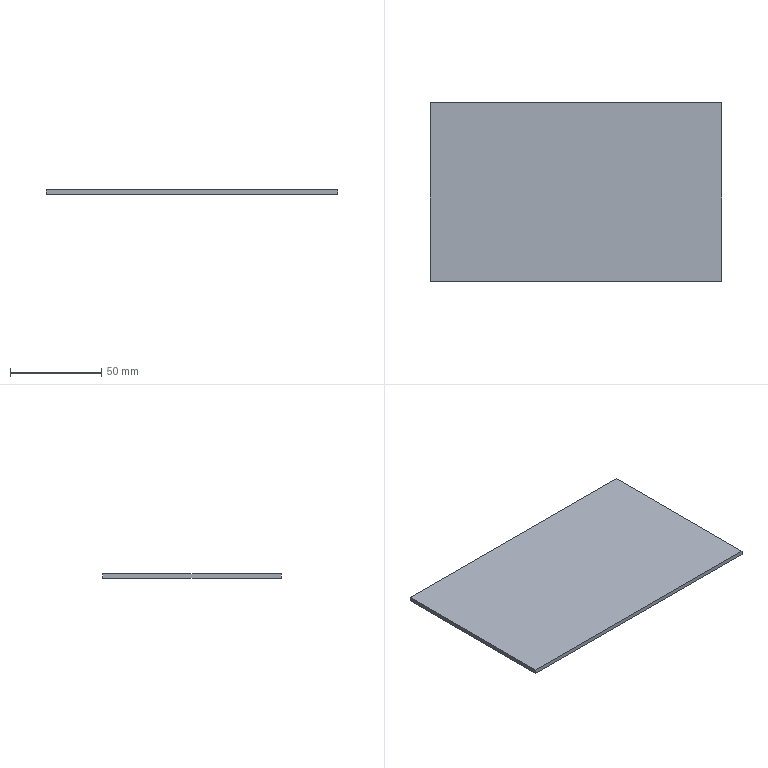Part | SolidWorks | features FlatPattern 1, SMBaseFlange 1, SheetMetal 1 | 1 solid | 6 faces | box 160 x 97.8 x 2.3 mm | volume 35990 mm3 | plane 6
STEP:
#1=CARTESIAN_POINT('',(0.,0.,0.));
#2=VERTEX_POINT('',#1);
#3=CARTESIAN_POINT('',(0.,-97.8,0.));
#4=VERTEX_POINT('',#3);
#5=CARTESIAN_POINT('',(0.,0.,0.));
#6=DIRECTION('',(0.,-1.,0.));
#7=VECTOR('',#6,1000.);
#8=LINE('',#5,#7);
#9=EDGE_CURVE('',#2,#4,#8,.T.);
#10=ORIENTED_EDGE('',*,*,#9,.F.);
#11=CARTESIAN_POINT('',(0.,0.,-2.3));
#12=VERTEX_POINT('',#11);
#13=CARTESIAN_POINT('',(0.,0.,-2.3));
#14=DIRECTION('',(0.,0.,1.));
#15=VECTOR('',#14,1000.);
#16=LINE('',#13,#15);
#17=EDGE_CURVE('',#12,#2,#16,.T.);
#18=ORIENTED_EDGE('',*,*,#17,.F.);
#19=CARTESIAN_POINT('',(0.,-97.8,-2.3));
#20=VERTEX_POINT('',#19);
#21=CARTESIAN_POINT('',(0.,0.,-2.3));
#22=DIRECTION('',(0.,-1.,0.));
#23=VECTOR('',#22,1000.);
#24=LINE('',#21,#23);
#25=EDGE_CURVE('',#12,#20,#24,.T.);
#26=ORIENTED_EDGE('',*,*,#25,.T.);
#27=CARTESIAN_POINT('',(0.,-97.8,-2.3));
#28=DIRECTION('',(0.,0.,1.));
#29=VECTOR('',#28,1000.);
#30=LINE('',#27,#29);
#31=EDGE_CURVE('',#20,#4,#30,.T.);
#32=ORIENTED_EDGE('',*,*,#31,.T.);
#33=EDGE_LOOP('',(#10,#18,#26,#32));
#34=FACE_OUTER_BOUND('',#33,.T.);
#35=CARTESIAN_POINT('',(0.,0.,-2.3));
#36=DIRECTION('',(-1.,0.,0.));
#37=DIRECTION('',(0.,-1.,0.));
#38=AXIS2_PLACEMENT_3D('',#35,#36,#37);
#39=PLANE('',#38);
#40=ADVANCED_FACE('',(#34),#39,.T.);
#41=CARTESIAN_POINT('',(160.,0.,0.));
#42=VERTEX_POINT('',#41);
#43=CARTESIAN_POINT('',(0.,0.,0.));
#44=DIRECTION('',(-1.,0.,0.));
#45=VECTOR('',#44,1000.);
#46=LINE('',#43,#45);
#47=EDGE_CURVE('',#42,#2,#46,.T.);
#48=ORIENTED_EDGE('',*,*,#47,.F.);
#49=CARTESIAN_POINT('',(160.,0.,-2.3));
#50=VERTEX_POINT('',#49);
#51=CARTESIAN_POINT('',(160.,0.,-2.3));
#52=DIRECTION('',(0.,0.,1.));
#53=VECTOR('',#52,1000.);
#54=LINE('',#51,#53);
#55=EDGE_CURVE('',#50,#42,#54,.T.);
#56=ORIENTED_EDGE('',*,*,#55,.F.);
#57=CARTESIAN_POINT('',(0.,0.,-2.3));
#58=DIRECTION('',(-1.,0.,0.));
#59=VECTOR('',#58,1000.);
#60=LINE('',#57,#59);
#61=EDGE_CURVE('',#50,#12,#60,.T.);
#62=ORIENTED_EDGE('',*,*,#61,.T.);
#63=ORIENTED_EDGE('',*,*,#17,.T.);
#64=EDGE_LOOP('',(#48,#56,#62,#63));
#65=FACE_OUTER_BOUND('',#64,.T.);
#66=CARTESIAN_POINT('',(0.,0.,-2.3));
#67=DIRECTION('',(0.,1.,0.));
#68=DIRECTION('',(0.,0.,1.));
#69=AXIS2_PLACEMENT_3D('',#66,#67,#68);
#70=PLANE('',#69);
#71=ADVANCED_FACE('',(#65),#70,.T.);
#72=CARTESIAN_POINT('',(160.,-97.8,0.));
#73=VERTEX_POINT('',#72);
#74=CARTESIAN_POINT('',(160.,0.,0.));
#75=DIRECTION('',(0.,1.,0.));
#76=VECTOR('',#75,1000.);
#77=LINE('',#74,#76);
#78=EDGE_CURVE('',#73,#42,#77,.T.);
#79=ORIENTED_EDGE('',*,*,#78,.F.);
#80=CARTESIAN_POINT('',(160.,-97.8,-2.3));
#81=VERTEX_POINT('',#80);
#82=CARTESIAN_POINT('',(160.,-97.8,-2.3));
#83=DIRECTION('',(0.,0.,1.));
#84=VECTOR('',#83,1000.);
#85=LINE('',#82,#84);
#86=EDGE_CURVE('',#81,#73,#85,.T.);
#87=ORIENTED_EDGE('',*,*,#86,.F.);
#88=CARTESIAN_POINT('',(160.,0.,-2.3));
#89=DIRECTION('',(0.,1.,0.));
#90=VECTOR('',#89,1000.);
#91=LINE('',#88,#90);
#92=EDGE_CURVE('',#81,#50,#91,.T.);
#93=ORIENTED_EDGE('',*,*,#92,.T.);
#94=ORIENTED_EDGE('',*,*,#55,.T.);
#95=EDGE_LOOP('',(#79,#87,#93,#94));
#96=FACE_OUTER_BOUND('',#95,.T.);
#97=CARTESIAN_POINT('',(160.,0.,-2.3));
#98=DIRECTION('',(1.,0.,0.));
#99=DIRECTION('',(0.,0.,-1.));
#100=AXIS2_PLACEMENT_3D('',#97,#98,#99);
#101=PLANE('',#100);
#102=ADVANCED_FACE('',(#96),#101,.T.);
#103=CARTESIAN_POINT('',(0.,-97.8,0.));
#104=DIRECTION('',(1.,0.,0.));
#105=VECTOR('',#104,1000.);
#106=LINE('',#103,#105);
#107=EDGE_CURVE('',#4,#73,#106,.T.);
#108=ORIENTED_EDGE('',*,*,#107,.F.);
#109=ORIENTED_EDGE('',*,*,#31,.F.);
#110=CARTESIAN_POINT('',(0.,-97.8,-2.3));
#111=DIRECTION('',(1.,0.,0.));
#112=VECTOR('',#111,1000.);
#113=LINE('',#110,#112);
#114=EDGE_CURVE('',#20,#81,#113,.T.);
#115=ORIENTED_EDGE('',*,*,#114,.T.);
#116=ORIENTED_EDGE('',*,*,#86,.T.);
#117=EDGE_LOOP('',(#108,#109,#115,#116));
#118=FACE_OUTER_BOUND('',#117,.T.);
#119=CARTESIAN_POINT('',(0.,-97.8,-2.3));
#120=DIRECTION('',(0.,-1.,0.));
#121=DIRECTION('',(0.,0.,-1.));
#122=AXIS2_PLACEMENT_3D('',#119,#120,#121);
#123=PLANE('',#122);
#124=ADVANCED_FACE('',(#118),#123,.T.);
#125=ORIENTED_EDGE('',*,*,#25,.F.);
#126=ORIENTED_EDGE('',*,*,#61,.F.);
#127=ORIENTED_EDGE('',*,*,#92,.F.);
#128=ORIENTED_EDGE('',*,*,#114,.F.);
#129=EDGE_LOOP('',(#125,#126,#127,#128));
#130=FACE_OUTER_BOUND('',#129,.T.);
#131=CARTESIAN_POINT('',(0.,0.,-2.3));
#132=DIRECTION('',(0.,0.,1.));
#133=DIRECTION('',(1.,0.,0.));
#134=AXIS2_PLACEMENT_3D('',#131,#132,#133);
#135=PLANE('',#134);
#136=ADVANCED_FACE('',(#130),#135,.F.);
#137=ORIENTED_EDGE('',*,*,#9,.T.);
#138=ORIENTED_EDGE('',*,*,#107,.T.);
#139=ORIENTED_EDGE('',*,*,#78,.T.);
#140=ORIENTED_EDGE('',*,*,#47,.T.);
#141=EDGE_LOOP('',(#137,#138,#139,#140));
#142=FACE_OUTER_BOUND('',#141,.T.);
#143=CARTESIAN_POINT('',(0.,0.,0.));
#144=DIRECTION('',(0.,0.,1.));
#145=DIRECTION('',(1.,0.,0.));
#146=AXIS2_PLACEMENT_3D('',#143,#144,#145);
#147=PLANE('',#146);
#148=ADVANCED_FACE('',(#142),#147,.T.);
#149=CLOSED_SHELL('',(#40,#71,#102,#124,#136,#148));
#150=MANIFOLD_SOLID_BREP('',#149);
#151=CARTESIAN_POINT('',(0.,0.,0.));
#152=DIRECTION('',(0.,0.,1.));
#153=DIRECTION('',(1.,0.,0.));
#154=AXIS2_PLACEMENT_3D('',#151,#152,#153);
#155=(LENGTH_UNIT()NAMED_UNIT(*)SI_UNIT(.MILLI.,.METRE.));
#156=UNCERTAINTY_MEASURE_WITH_UNIT(LENGTH_MEASURE(0.00001),#155,'','');
#157=(NAMED_UNIT(*)PLANE_ANGLE_UNIT()SI_UNIT($,.RADIAN.));
#158=(NAMED_UNIT(*)SI_UNIT($,.STERADIAN.)SOLID_ANGLE_UNIT());
#159=(GEOMETRIC_REPRESENTATION_CONTEXT(3)GLOBAL_UNCERTAINTY_ASSIGNED_CONTEXT((#156))GLOBAL_UNIT_ASSIGNED_CONTEXT((#155,#157,#158))REPRESENTATION_CONTEXT('',''));
#160=ADVANCED_BREP_SHAPE_REPRESENTATION('',(#150,#154),#159);